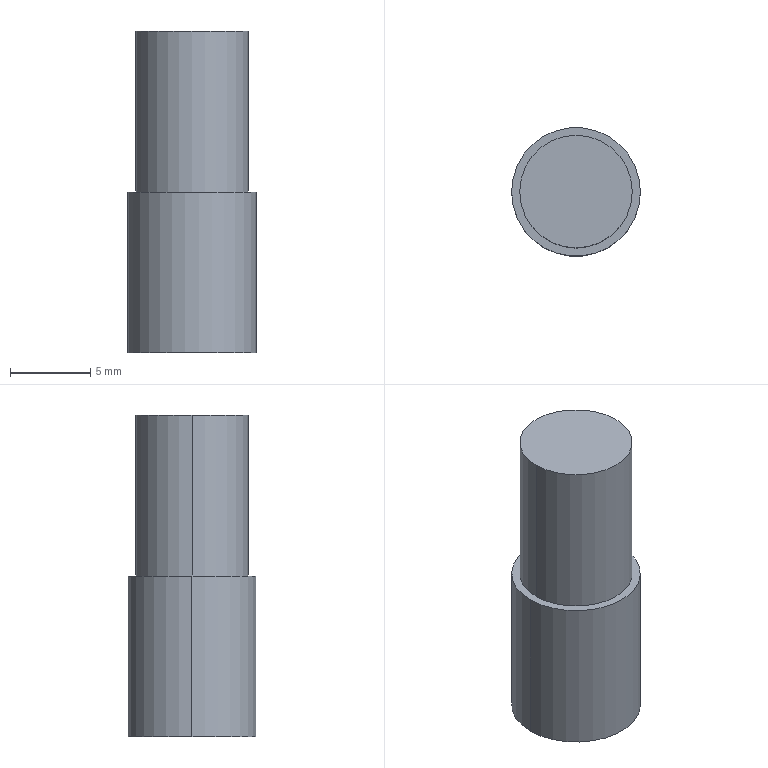Part | STEP file | Distributor part locating pin SGN-2-25 | 1 solid | 7 faces | box 8 x 8 x 20 mm | volume 887.5 mm3 | cylinder 4 | plane 3 | commonest cylinder face diameters 7 x2 8 x2
STEP:
#1=CARTESIAN_POINT('',(0.,0.,0.));
#2=DIRECTION('',(0.,0.,1.));
#3=DIRECTION('',(1.,0.,0.));
#4=AXIS2_PLACEMENT_3D('',#1,#2,#3);
#5=CARTESIAN_POINT('',(-4.,0.,-10.));
#6=VERTEX_POINT('',#5);
#7=CARTESIAN_POINT('',(4.,0.,-10.));
#8=VERTEX_POINT('',#7);
#9=CARTESIAN_POINT('',(0.,0.,-10.));
#10=DIRECTION('',(0.,0.,-1.));
#11=DIRECTION('',(-1.,0.,0.));
#12=AXIS2_PLACEMENT_3D('',#9,#10,#11);
#13=CIRCLE('',#12,4.);
#14=CARTESIAN_POINT('',(0.,0.,-10.));
#15=DIRECTION('',(0.,0.,1.));
#16=DIRECTION('',(1.,0.,0.));
#17=AXIS2_PLACEMENT_3D('',#14,#15,#16);
#18=CYLINDRICAL_SURFACE('',#17,4.);
#19=CARTESIAN_POINT('',(3.142,0.));
#20=DIRECTION('',(-1.,0.));
#21=VECTOR('',#20,1.);
#22=LINE('',#19,#21);
#23=(GEOMETRIC_REPRESENTATION_CONTEXT(2)PARAMETRIC_REPRESENTATION_CONTEXT()REPRESENTATION_CONTEXT('',''));
#24=DEFINITIONAL_REPRESENTATION('',(#22),#23);
#25=PCURVE('',#18,#24);
#26=CARTESIAN_POINT('',(0.,0.,-10.));
#27=DIRECTION('',(0.,0.,-1.));
#28=DIRECTION('',(-1.,0.,0.));
#29=AXIS2_PLACEMENT_3D('',#26,#27,#28);
#30=PLANE('',#29);
#31=CARTESIAN_POINT('',(0.,0.));
#32=DIRECTION('',(1.,0.));
#33=AXIS2_PLACEMENT_2D('',#31,#32);
#34=CIRCLE('',#33,4.);
#35=(GEOMETRIC_REPRESENTATION_CONTEXT(2)PARAMETRIC_REPRESENTATION_CONTEXT()REPRESENTATION_CONTEXT('',''));
#36=DEFINITIONAL_REPRESENTATION('',(#34),#35);
#37=PCURVE('',#30,#36);
#38=SURFACE_CURVE('',#13,(#25,#37),.PCURVE_S1.);
#39=EDGE_CURVE('',#6,#8,#38,.T.);
#40=ORIENTED_EDGE('',*,*,#39,.F.);
#41=CARTESIAN_POINT('',(-4.,0.,0.));
#42=VERTEX_POINT('',#41);
#43=CARTESIAN_POINT('',(-4.,0.,-10.));
#44=DIRECTION('',(0.,0.,1.));
#45=VECTOR('',#44,1.);
#46=LINE('',#43,#45);
#47=CARTESIAN_POINT('',(3.142,0.));
#48=DIRECTION('',(0.,1.));
#49=VECTOR('',#48,1.);
#50=LINE('',#47,#49);
#51=(GEOMETRIC_REPRESENTATION_CONTEXT(2)PARAMETRIC_REPRESENTATION_CONTEXT()REPRESENTATION_CONTEXT('',''));
#52=DEFINITIONAL_REPRESENTATION('',(#50),#51);
#53=PCURVE('',#18,#52);
#54=CARTESIAN_POINT('',(0.,0.,-10.));
#55=DIRECTION('',(0.,0.,1.));
#56=DIRECTION('',(1.,0.,0.));
#57=AXIS2_PLACEMENT_3D('',#54,#55,#56);
#58=CYLINDRICAL_SURFACE('',#57,4.);
#59=CARTESIAN_POINT('',(3.142,0.));
#60=DIRECTION('',(0.,1.));
#61=VECTOR('',#60,1.);
#62=LINE('',#59,#61);
#63=(GEOMETRIC_REPRESENTATION_CONTEXT(2)PARAMETRIC_REPRESENTATION_CONTEXT()REPRESENTATION_CONTEXT('',''));
#64=DEFINITIONAL_REPRESENTATION('',(#62),#63);
#65=PCURVE('',#58,#64);
#66=SURFACE_CURVE('',#46,(#53,#65),.PCURVE_S1.);
#67=EDGE_CURVE('',#6,#42,#66,.T.);
#68=ORIENTED_EDGE('',*,*,#67,.T.);
#69=CARTESIAN_POINT('',(4.,0.,0.));
#70=VERTEX_POINT('',#69);
#71=CARTESIAN_POINT('',(0.,0.,0.));
#72=DIRECTION('',(0.,0.,-1.));
#73=DIRECTION('',(-1.,0.,0.));
#74=AXIS2_PLACEMENT_3D('',#71,#72,#73);
#75=CIRCLE('',#74,4.);
#76=CARTESIAN_POINT('',(3.142,10.));
#77=DIRECTION('',(-1.,0.));
#78=VECTOR('',#77,1.);
#79=LINE('',#76,#78);
#80=(GEOMETRIC_REPRESENTATION_CONTEXT(2)PARAMETRIC_REPRESENTATION_CONTEXT()REPRESENTATION_CONTEXT('',''));
#81=DEFINITIONAL_REPRESENTATION('',(#79),#80);
#82=PCURVE('',#18,#81);
#83=CARTESIAN_POINT('',(0.,0.,0.));
#84=DIRECTION('',(0.,0.,-1.));
#85=DIRECTION('',(-1.,0.,0.));
#86=AXIS2_PLACEMENT_3D('',#83,#84,#85);
#87=PLANE('',#86);
#88=CARTESIAN_POINT('',(0.,0.));
#89=DIRECTION('',(1.,0.));
#90=AXIS2_PLACEMENT_2D('',#88,#89);
#91=CIRCLE('',#90,4.);
#92=(GEOMETRIC_REPRESENTATION_CONTEXT(2)PARAMETRIC_REPRESENTATION_CONTEXT()REPRESENTATION_CONTEXT('',''));
#93=DEFINITIONAL_REPRESENTATION('',(#91),#92);
#94=PCURVE('',#87,#93);
#95=SURFACE_CURVE('',#75,(#82,#94),.PCURVE_S1.);
#96=EDGE_CURVE('',#42,#70,#95,.T.);
#97=ORIENTED_EDGE('',*,*,#96,.T.);
#98=CARTESIAN_POINT('',(4.,0.,-10.));
#99=DIRECTION('',(0.,0.,1.));
#100=VECTOR('',#99,1.);
#101=LINE('',#98,#100);
#102=CARTESIAN_POINT('',(0.,0.));
#103=DIRECTION('',(0.,1.));
#104=VECTOR('',#103,1.);
#105=LINE('',#102,#104);
#106=(GEOMETRIC_REPRESENTATION_CONTEXT(2)PARAMETRIC_REPRESENTATION_CONTEXT()REPRESENTATION_CONTEXT('',''));
#107=DEFINITIONAL_REPRESENTATION('',(#105),#106);
#108=PCURVE('',#18,#107);
#109=CARTESIAN_POINT('',(6.283,0.));
#110=DIRECTION('',(0.,1.));
#111=VECTOR('',#110,1.);
#112=LINE('',#109,#111);
#113=(GEOMETRIC_REPRESENTATION_CONTEXT(2)PARAMETRIC_REPRESENTATION_CONTEXT()REPRESENTATION_CONTEXT('',''));
#114=DEFINITIONAL_REPRESENTATION('',(#112),#113);
#115=PCURVE('',#58,#114);
#116=SURFACE_CURVE('',#101,(#108,#115),.PCURVE_S1.);
#117=EDGE_CURVE('',#8,#70,#116,.T.);
#118=ORIENTED_EDGE('',*,*,#117,.F.);
#119=EDGE_LOOP('',(#40,#68,#97,#118));
#120=FACE_BOUND('',#119,.T.);
#121=ADVANCED_FACE('',(#120),#18,.T.);
#122=CARTESIAN_POINT('',(3.5,0.,10.));
#123=VERTEX_POINT('',#122);
#124=CARTESIAN_POINT('',(-3.5,0.,10.));
#125=VERTEX_POINT('',#124);
#126=CARTESIAN_POINT('',(0.,0.,10.));
#127=DIRECTION('',(0.,0.,1.));
#128=DIRECTION('',(1.,0.,0.));
#129=AXIS2_PLACEMENT_3D('',#126,#127,#128);
#130=CIRCLE('',#129,3.5);
#131=CARTESIAN_POINT('',(0.,0.,10.));
#132=DIRECTION('',(0.,0.,-1.));
#133=DIRECTION('',(-1.,0.,0.));
#134=AXIS2_PLACEMENT_3D('',#131,#132,#133);
#135=CYLINDRICAL_SURFACE('',#134,3.5);
#136=CARTESIAN_POINT('',(3.142,0.));
#137=DIRECTION('',(-1.,0.));
#138=VECTOR('',#137,1.);
#139=LINE('',#136,#138);
#140=(GEOMETRIC_REPRESENTATION_CONTEXT(2)PARAMETRIC_REPRESENTATION_CONTEXT()REPRESENTATION_CONTEXT('',''));
#141=DEFINITIONAL_REPRESENTATION('',(#139),#140);
#142=PCURVE('',#135,#141);
#143=CARTESIAN_POINT('',(0.,0.,10.));
#144=DIRECTION('',(0.,0.,1.));
#145=DIRECTION('',(1.,0.,0.));
#146=AXIS2_PLACEMENT_3D('',#143,#144,#145);
#147=PLANE('',#146);
#148=CARTESIAN_POINT('',(0.,0.));
#149=DIRECTION('',(1.,0.));
#150=AXIS2_PLACEMENT_2D('',#148,#149);
#151=CIRCLE('',#150,3.5);
#152=(GEOMETRIC_REPRESENTATION_CONTEXT(2)PARAMETRIC_REPRESENTATION_CONTEXT()REPRESENTATION_CONTEXT('',''));
#153=DEFINITIONAL_REPRESENTATION('',(#151),#152);
#154=PCURVE('',#147,#153);
#155=SURFACE_CURVE('',#130,(#142,#154),.PCURVE_S1.);
#156=EDGE_CURVE('',#123,#125,#155,.T.);
#157=ORIENTED_EDGE('',*,*,#156,.F.);
#158=CARTESIAN_POINT('',(3.5,0.,0.));
#159=VERTEX_POINT('',#158);
#160=CARTESIAN_POINT('',(3.5,0.,10.));
#161=DIRECTION('',(0.,0.,-1.));
#162=VECTOR('',#161,1.);
#163=LINE('',#160,#162);
#164=CARTESIAN_POINT('',(3.142,0.));
#165=DIRECTION('',(0.,1.));
#166=VECTOR('',#165,1.);
#167=LINE('',#164,#166);
#168=(GEOMETRIC_REPRESENTATION_CONTEXT(2)PARAMETRIC_REPRESENTATION_CONTEXT()REPRESENTATION_CONTEXT('',''));
#169=DEFINITIONAL_REPRESENTATION('',(#167),#168);
#170=PCURVE('',#135,#169);
#171=CARTESIAN_POINT('',(0.,0.,10.));
#172=DIRECTION('',(0.,0.,-1.));
#173=DIRECTION('',(-1.,0.,0.));
#174=AXIS2_PLACEMENT_3D('',#171,#172,#173);
#175=CYLINDRICAL_SURFACE('',#174,3.5);
#176=CARTESIAN_POINT('',(3.142,0.));
#177=DIRECTION('',(0.,1.));
#178=VECTOR('',#177,1.);
#179=LINE('',#176,#178);
#180=(GEOMETRIC_REPRESENTATION_CONTEXT(2)PARAMETRIC_REPRESENTATION_CONTEXT()REPRESENTATION_CONTEXT('',''));
#181=DEFINITIONAL_REPRESENTATION('',(#179),#180);
#182=PCURVE('',#175,#181);
#183=SURFACE_CURVE('',#163,(#170,#182),.PCURVE_S1.);
#184=EDGE_CURVE('',#123,#159,#183,.T.);
#185=ORIENTED_EDGE('',*,*,#184,.T.);
#186=CARTESIAN_POINT('',(-3.5,0.,0.));
#187=VERTEX_POINT('',#186);
#188=CARTESIAN_POINT('',(0.,0.,0.));
#189=DIRECTION('',(0.,0.,1.));
#190=DIRECTION('',(1.,0.,0.));
#191=AXIS2_PLACEMENT_3D('',#188,#189,#190);
#192=CIRCLE('',#191,3.5);
#193=CARTESIAN_POINT('',(3.142,10.));
#194=DIRECTION('',(-1.,0.));
#195=VECTOR('',#194,1.);
#196=LINE('',#193,#195);
#197=(GEOMETRIC_REPRESENTATION_CONTEXT(2)PARAMETRIC_REPRESENTATION_CONTEXT()REPRESENTATION_CONTEXT('',''));
#198=DEFINITIONAL_REPRESENTATION('',(#196),#197);
#199=PCURVE('',#135,#198);
#200=CARTESIAN_POINT('',(-3.5,0.));
#201=CARTESIAN_POINT('',(-3.5,6.062));
#202=CARTESIAN_POINT('',(1.75,3.031));
#203=CARTESIAN_POINT('',(7.,0.));
#204=CARTESIAN_POINT('',(1.75,-3.031));
#205=CARTESIAN_POINT('',(-3.5,-6.062));
#206=CARTESIAN_POINT('',(-3.5,0.));
#207=(BOUNDED_CURVE()B_SPLINE_CURVE(2,(#200,#201,#202,#203,#204,#205,#206),.UNSPECIFIED.,.T.,.F.)B_SPLINE_CURVE_WITH_KNOTS((1,2,2,2,2,1),(-2.094,0.,2.094,4.189,6.283,8.378),.UNSPECIFIED.)CURVE()GEOMETRIC_REPRESENTATION_ITEM()RATIONAL_B_SPLINE_CURVE((1.,0.5,1.,0.5,1.,0.5,1.))REPRESENTATION_ITEM(''));
#208=(GEOMETRIC_REPRESENTATION_CONTEXT(2)PARAMETRIC_REPRESENTATION_CONTEXT()REPRESENTATION_CONTEXT('',''));
#209=DEFINITIONAL_REPRESENTATION('',(#207),#208);
#210=PCURVE('',#87,#209);
#211=SURFACE_CURVE('',#192,(#199,#210),.PCURVE_S1.);
#212=EDGE_CURVE('',#159,#187,#211,.T.);
#213=ORIENTED_EDGE('',*,*,#212,.T.);
#214=CARTESIAN_POINT('',(-3.5,0.,10.));
#215=DIRECTION('',(0.,0.,-1.));
#216=VECTOR('',#215,1.);
#217=LINE('',#214,#216);
#218=CARTESIAN_POINT('',(0.,0.));
#219=DIRECTION('',(0.,1.));
#220=VECTOR('',#219,1.);
#221=LINE('',#218,#220);
#222=(GEOMETRIC_REPRESENTATION_CONTEXT(2)PARAMETRIC_REPRESENTATION_CONTEXT()REPRESENTATION_CONTEXT('',''));
#223=DEFINITIONAL_REPRESENTATION('',(#221),#222);
#224=PCURVE('',#135,#223);
#225=CARTESIAN_POINT('',(6.283,0.));
#226=DIRECTION('',(0.,1.));
#227=VECTOR('',#226,1.);
#228=LINE('',#225,#227);
#229=(GEOMETRIC_REPRESENTATION_CONTEXT(2)PARAMETRIC_REPRESENTATION_CONTEXT()REPRESENTATION_CONTEXT('',''));
#230=DEFINITIONAL_REPRESENTATION('',(#228),#229);
#231=PCURVE('',#175,#230);
#232=SURFACE_CURVE('',#217,(#224,#231),.PCURVE_S1.);
#233=EDGE_CURVE('',#125,#187,#232,.T.);
#234=ORIENTED_EDGE('',*,*,#233,.F.);
#235=EDGE_LOOP('',(#157,#185,#213,#234));
#236=FACE_BOUND('',#235,.T.);
#237=ADVANCED_FACE('',(#236),#135,.T.);
#238=ORIENTED_EDGE('',*,*,#184,.F.);
#239=CARTESIAN_POINT('',(0.,0.,10.));
#240=DIRECTION('',(0.,0.,1.));
#241=DIRECTION('',(1.,0.,0.));
#242=AXIS2_PLACEMENT_3D('',#239,#240,#241);
#243=CIRCLE('',#242,3.5);
#244=CARTESIAN_POINT('',(9.425,0.));
#245=DIRECTION('',(-1.,0.));
#246=VECTOR('',#245,1.);
#247=LINE('',#244,#246);
#248=(GEOMETRIC_REPRESENTATION_CONTEXT(2)PARAMETRIC_REPRESENTATION_CONTEXT()REPRESENTATION_CONTEXT('',''));
#249=DEFINITIONAL_REPRESENTATION('',(#247),#248);
#250=PCURVE('',#175,#249);
#251=CARTESIAN_POINT('',(0.,0.));
#252=DIRECTION('',(1.,0.));
#253=AXIS2_PLACEMENT_2D('',#251,#252);
#254=CIRCLE('',#253,3.5);
#255=(GEOMETRIC_REPRESENTATION_CONTEXT(2)PARAMETRIC_REPRESENTATION_CONTEXT()REPRESENTATION_CONTEXT('',''));
#256=DEFINITIONAL_REPRESENTATION('',(#254),#255);
#257=PCURVE('',#147,#256);
#258=SURFACE_CURVE('',#243,(#250,#257),.PCURVE_S1.);
#259=EDGE_CURVE('',#125,#123,#258,.T.);
#260=ORIENTED_EDGE('',*,*,#259,.F.);
#261=ORIENTED_EDGE('',*,*,#233,.T.);
#262=CARTESIAN_POINT('',(0.,0.,0.));
#263=DIRECTION('',(0.,0.,1.));
#264=DIRECTION('',(1.,0.,0.));
#265=AXIS2_PLACEMENT_3D('',#262,#263,#264);
#266=CIRCLE('',#265,3.5);
#267=CARTESIAN_POINT('',(9.425,10.));
#268=DIRECTION('',(-1.,0.));
#269=VECTOR('',#268,1.);
#270=LINE('',#267,#269);
#271=(GEOMETRIC_REPRESENTATION_CONTEXT(2)PARAMETRIC_REPRESENTATION_CONTEXT()REPRESENTATION_CONTEXT('',''));
#272=DEFINITIONAL_REPRESENTATION('',(#270),#271);
#273=PCURVE('',#175,#272);
#274=CARTESIAN_POINT('',(-3.5,0.));
#275=CARTESIAN_POINT('',(-3.5,6.062));
#276=CARTESIAN_POINT('',(1.75,3.031));
#277=CARTESIAN_POINT('',(7.,0.));
#278=CARTESIAN_POINT('',(1.75,-3.031));
#279=CARTESIAN_POINT('',(-3.5,-6.062));
#280=CARTESIAN_POINT('',(-3.5,0.));
#281=(BOUNDED_CURVE()B_SPLINE_CURVE(2,(#274,#275,#276,#277,#278,#279,#280),.UNSPECIFIED.,.T.,.F.)B_SPLINE_CURVE_WITH_KNOTS((1,2,2,2,2,1),(-2.094,0.,2.094,4.189,6.283,8.378),.UNSPECIFIED.)CURVE()GEOMETRIC_REPRESENTATION_ITEM()RATIONAL_B_SPLINE_CURVE((1.,0.5,1.,0.5,1.,0.5,1.))REPRESENTATION_ITEM(''));
#282=(GEOMETRIC_REPRESENTATION_CONTEXT(2)PARAMETRIC_REPRESENTATION_CONTEXT()REPRESENTATION_CONTEXT('',''));
#283=DEFINITIONAL_REPRESENTATION('',(#281),#282);
#284=PCURVE('',#87,#283);
#285=SURFACE_CURVE('',#266,(#273,#284),.PCURVE_S1.);
#286=EDGE_CURVE('',#187,#159,#285,.T.);
#287=ORIENTED_EDGE('',*,*,#286,.T.);
#288=EDGE_LOOP('',(#238,#260,#261,#287));
#289=FACE_BOUND('',#288,.T.);
#290=ADVANCED_FACE('',(#289),#175,.T.);
#291=ORIENTED_EDGE('',*,*,#259,.T.);
#292=ORIENTED_EDGE('',*,*,#156,.T.);
#293=EDGE_LOOP('',(#291,#292));
#294=FACE_BOUND('',#293,.T.);
#295=ADVANCED_FACE('',(#294),#147,.T.);
#296=ORIENTED_EDGE('',*,*,#67,.F.);
#297=CARTESIAN_POINT('',(0.,0.,-10.));
#298=DIRECTION('',(0.,0.,-1.));
#299=DIRECTION('',(-1.,0.,0.));
#300=AXIS2_PLACEMENT_3D('',#297,#298,#299);
#301=CIRCLE('',#300,4.);
#302=CARTESIAN_POINT('',(9.425,0.));
#303=DIRECTION('',(-1.,0.));
#304=VECTOR('',#303,1.);
#305=LINE('',#302,#304);
#306=(GEOMETRIC_REPRESENTATION_CONTEXT(2)PARAMETRIC_REPRESENTATION_CONTEXT()REPRESENTATION_CONTEXT('',''));
#307=DEFINITIONAL_REPRESENTATION('',(#305),#306);
#308=PCURVE('',#58,#307);
#309=CARTESIAN_POINT('',(0.,0.));
#310=DIRECTION('',(1.,0.));
#311=AXIS2_PLACEMENT_2D('',#309,#310);
#312=CIRCLE('',#311,4.);
#313=(GEOMETRIC_REPRESENTATION_CONTEXT(2)PARAMETRIC_REPRESENTATION_CONTEXT()REPRESENTATION_CONTEXT('',''));
#314=DEFINITIONAL_REPRESENTATION('',(#312),#313);
#315=PCURVE('',#30,#314);
#316=SURFACE_CURVE('',#301,(#308,#315),.PCURVE_S1.);
#317=EDGE_CURVE('',#8,#6,#316,.T.);
#318=ORIENTED_EDGE('',*,*,#317,.F.);
#319=ORIENTED_EDGE('',*,*,#117,.T.);
#320=CARTESIAN_POINT('',(0.,0.,0.));
#321=DIRECTION('',(0.,0.,-1.));
#322=DIRECTION('',(-1.,0.,0.));
#323=AXIS2_PLACEMENT_3D('',#320,#321,#322);
#324=CIRCLE('',#323,4.);
#325=CARTESIAN_POINT('',(9.425,10.));
#326=DIRECTION('',(-1.,0.));
#327=VECTOR('',#326,1.);
#328=LINE('',#325,#327);
#329=(GEOMETRIC_REPRESENTATION_CONTEXT(2)PARAMETRIC_REPRESENTATION_CONTEXT()REPRESENTATION_CONTEXT('',''));
#330=DEFINITIONAL_REPRESENTATION('',(#328),#329);
#331=PCURVE('',#58,#330);
#332=CARTESIAN_POINT('',(0.,0.));
#333=DIRECTION('',(1.,0.));
#334=AXIS2_PLACEMENT_2D('',#332,#333);
#335=CIRCLE('',#334,4.);
#336=(GEOMETRIC_REPRESENTATION_CONTEXT(2)PARAMETRIC_REPRESENTATION_CONTEXT()REPRESENTATION_CONTEXT('',''));
#337=DEFINITIONAL_REPRESENTATION('',(#335),#336);
#338=PCURVE('',#87,#337);
#339=SURFACE_CURVE('',#324,(#331,#338),.PCURVE_S1.);
#340=EDGE_CURVE('',#70,#42,#339,.T.);
#341=ORIENTED_EDGE('',*,*,#340,.T.);
#342=EDGE_LOOP('',(#296,#318,#319,#341));
#343=FACE_BOUND('',#342,.T.);
#344=ADVANCED_FACE('',(#343),#58,.T.);
#345=ORIENTED_EDGE('',*,*,#317,.T.);
#346=ORIENTED_EDGE('',*,*,#39,.T.);
#347=EDGE_LOOP('',(#345,#346));
#348=FACE_BOUND('',#347,.T.);
#349=ADVANCED_FACE('',(#348),#30,.T.);
#350=ORIENTED_EDGE('',*,*,#286,.F.);
#351=ORIENTED_EDGE('',*,*,#212,.F.);
#352=EDGE_LOOP('',(#350,#351));
#353=FACE_BOUND('',#352,.T.);
#354=ORIENTED_EDGE('',*,*,#340,.F.);
#355=ORIENTED_EDGE('',*,*,#96,.F.);
#356=EDGE_LOOP('',(#354,#355));
#357=FACE_BOUND('',#356,.T.);
#358=ADVANCED_FACE('',(#353,#357),#87,.F.);
#359=CLOSED_SHELL('',(#121,#237,#290,#295,#344,#349,#358));
#360=MANIFOLD_SOLID_BREP('',#359);
#361=(LENGTH_UNIT()NAMED_UNIT(*)SI_UNIT(.MILLI.,.METRE.));
#362=UNCERTAINTY_MEASURE_WITH_UNIT(LENGTH_MEASURE(0.0000001),#361,'','');
#363=(NAMED_UNIT(*)PLANE_ANGLE_UNIT()SI_UNIT($,.RADIAN.));
#364=(NAMED_UNIT(*)SI_UNIT($,.STERADIAN.)SOLID_ANGLE_UNIT());
#365=(GEOMETRIC_REPRESENTATION_CONTEXT(3)GLOBAL_UNCERTAINTY_ASSIGNED_CONTEXT((#362))GLOBAL_UNIT_ASSIGNED_CONTEXT((#361,#363,#364))REPRESENTATION_CONTEXT('',''));
#366=ADVANCED_BREP_SHAPE_REPRESENTATION('',(#4,#360),#365);